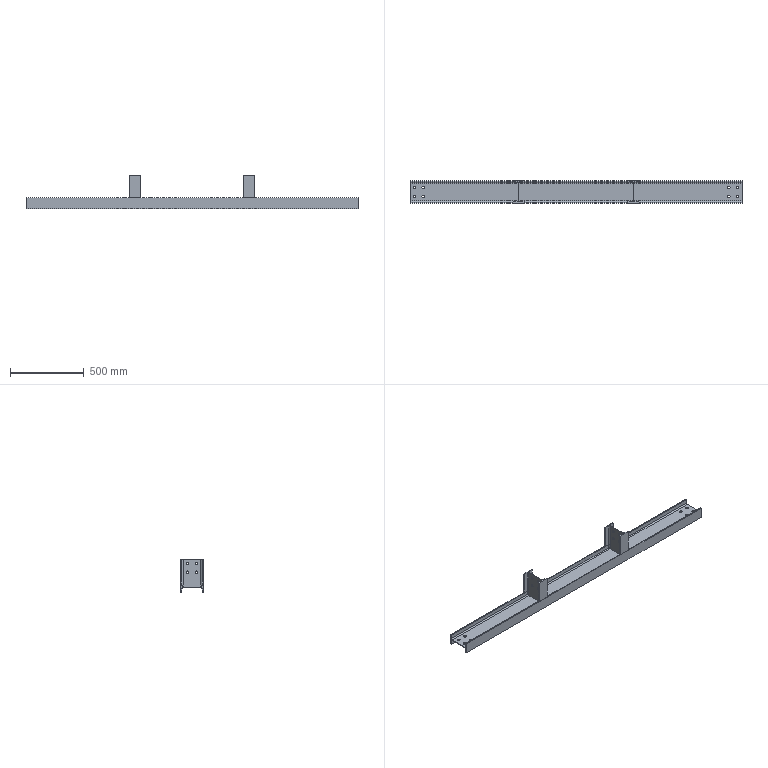Part | STEP file | 粉仓辅梁16主体_Default<As Machined> | 3 solids | 98 faces | box 2255 x 150 x 230 mm | volume 4605807 mm3 | plane 54 | cylinder 44 | commonest cylinder face diameters 19 x32 16 x12